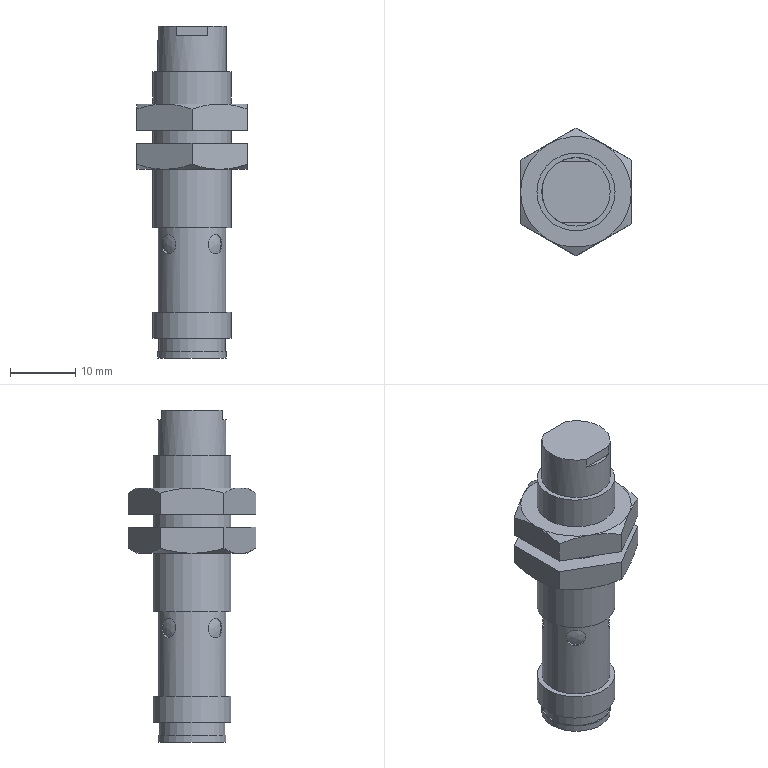Part | NX | 1 solid | 66 faces | box 17 x 19.63 x 51 mm | volume 5737 mm3 | plane 37 | cylinder 13 | cone 12 | sphere 4 | commonest cylinder face diameters 3 x4 12 x4 10.5 x2 8.3 x1 10.2 x1 10.4 x1